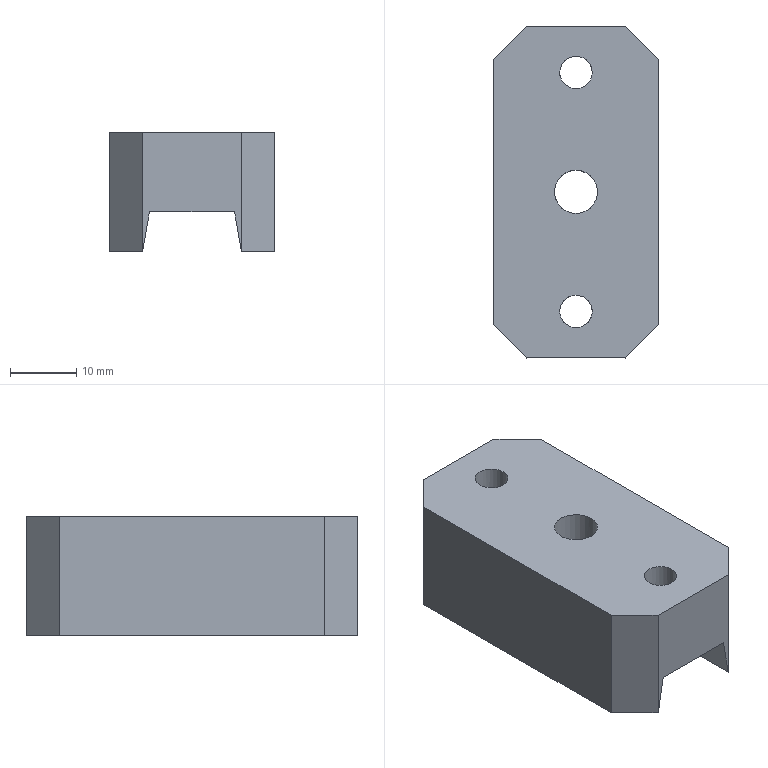Part | STEP file | 车灯-后视镜_id258_x_t | 1 solid | 19 faces | box 25 x 50 x 18 mm | volume 16008 mm3 | plane 15 | cylinder 4 | commonest cylinder face diameters 4.9 x2 6.5 x1 12.5 x1
STEP:
#1=CARTESIAN_POINT('',(-180.,153.25,17.94));
#2=VERTEX_POINT('',#1);
#3=CARTESIAN_POINT('',(-180.,150.,17.94));
#4=DIRECTION('',(0.,0.,-1.));
#5=DIRECTION('',(0.,1.,0.));
#6=AXIS2_PLACEMENT_3D('',#3,#4,#5);
#7=CIRCLE('',#6,3.25);
#8=EDGE_CURVE('',#2,#2,#7,.T.);
#9=ORIENTED_EDGE('',*,*,#8,.F.);
#10=EDGE_LOOP('',(#9));
#11=FACE_BOUND('',#10,.T.);
#12=CARTESIAN_POINT('',(-183.25,150.,12.44));
#13=VERTEX_POINT('',#12);
#14=CARTESIAN_POINT('',(-180.,150.,12.44));
#15=DIRECTION('',(0.,0.,1.));
#16=DIRECTION('',(-1.,0.,0.));
#17=AXIS2_PLACEMENT_3D('',#14,#15,#16);
#18=CIRCLE('',#17,3.25);
#19=EDGE_CURVE('',#13,#13,#18,.T.);
#20=ORIENTED_EDGE('',*,*,#19,.F.);
#21=EDGE_LOOP('',(#20));
#22=FACE_BOUND('',#21,.T.);
#23=CARTESIAN_POINT('',(-180.,150.,21.94));
#24=DIRECTION('',(0.,0.,-1.));
#25=DIRECTION('',(1.,0.,0.));
#26=AXIS2_PLACEMENT_3D('',#23,#24,#25);
#27=CYLINDRICAL_SURFACE('',#26,3.25);
#28=ADVANCED_FACE('',(#11,#22),#27,.F.);
#29=CARTESIAN_POINT('',(-172.5,125.,17.94));
#30=VERTEX_POINT('',#29);
#31=CARTESIAN_POINT('',(-187.5,125.,17.94));
#32=VERTEX_POINT('',#31);
#33=CARTESIAN_POINT('',(-195.,125.,17.94));
#34=DIRECTION('',(-1.,0.,0.));
#35=VECTOR('',#34,1.);
#36=LINE('',#33,#35);
#37=EDGE_CURVE('',#30,#32,#36,.T.);
#38=ORIENTED_EDGE('',*,*,#37,.T.);
#39=CARTESIAN_POINT('',(-187.5,125.,-0.05985));
#40=VERTEX_POINT('',#39);
#41=CARTESIAN_POINT('',(-187.5,125.,-0.05985));
#42=DIRECTION('',(0.,0.,-1.));
#43=VECTOR('',#42,1.);
#44=LINE('',#41,#43);
#45=EDGE_CURVE('',#32,#40,#44,.T.);
#46=ORIENTED_EDGE('',*,*,#45,.T.);
#47=CARTESIAN_POINT('',(-187.461,125.,-0.05985));
#48=VERTEX_POINT('',#47);
#49=CARTESIAN_POINT('',(-195.,125.,-0.05985));
#50=DIRECTION('',(-1.,0.,0.));
#51=VECTOR('',#50,1.);
#52=LINE('',#49,#51);
#53=EDGE_CURVE('',#48,#40,#52,.T.);
#54=ORIENTED_EDGE('',*,*,#53,.F.);
#55=CARTESIAN_POINT('',(-186.403,125.,5.94));
#56=VERTEX_POINT('',#55);
#57=CARTESIAN_POINT('',(-187.538,125.,-0.494));
#58=DIRECTION('',(-0.1736,0.,-0.9848));
#59=VECTOR('',#58,1.);
#60=LINE('',#57,#59);
#61=EDGE_CURVE('',#56,#48,#60,.T.);
#62=ORIENTED_EDGE('',*,*,#61,.F.);
#63=CARTESIAN_POINT('',(-173.597,125.,5.94));
#64=VERTEX_POINT('',#63);
#65=CARTESIAN_POINT('',(-172.5,125.,5.94));
#66=DIRECTION('',(-1.,0.,0.));
#67=VECTOR('',#66,1.);
#68=LINE('',#65,#67);
#69=EDGE_CURVE('',#64,#56,#68,.T.);
#70=ORIENTED_EDGE('',*,*,#69,.F.);
#71=CARTESIAN_POINT('',(-172.539,125.,-0.05985));
#72=VERTEX_POINT('',#71);
#73=CARTESIAN_POINT('',(-172.462,125.,-0.494));
#74=DIRECTION('',(0.1736,0.,-0.9848));
#75=VECTOR('',#74,1.);
#76=LINE('',#73,#75);
#77=EDGE_CURVE('',#64,#72,#76,.T.);
#78=ORIENTED_EDGE('',*,*,#77,.T.);
#79=CARTESIAN_POINT('',(-172.5,125.,-0.05985));
#80=VERTEX_POINT('',#79);
#81=CARTESIAN_POINT('',(-195.,125.,-0.05985));
#82=DIRECTION('',(-1.,0.,0.));
#83=VECTOR('',#82,1.);
#84=LINE('',#81,#83);
#85=EDGE_CURVE('',#80,#72,#84,.T.);
#86=ORIENTED_EDGE('',*,*,#85,.F.);
#87=CARTESIAN_POINT('',(-172.5,125.,-0.05985));
#88=DIRECTION('',(0.,0.,1.));
#89=VECTOR('',#88,1.);
#90=LINE('',#87,#89);
#91=EDGE_CURVE('',#80,#30,#90,.T.);
#92=ORIENTED_EDGE('',*,*,#91,.T.);
#93=EDGE_LOOP('',(#38,#46,#54,#62,#70,#78,#86,#92));
#94=FACE_OUTER_BOUND('',#93,.T.);
#95=CARTESIAN_POINT('',(-165.,125.,-0.05985));
#96=DIRECTION('',(0.,1.,0.));
#97=DIRECTION('',(1.,0.,0.));
#98=AXIS2_PLACEMENT_3D('',#95,#96,#97);
#99=PLANE('',#98);
#100=ADVANCED_FACE('',(#94),#99,.F.);
#101=CARTESIAN_POINT('',(-172.5,175.,17.94));
#102=VERTEX_POINT('',#101);
#103=CARTESIAN_POINT('',(-187.5,175.,17.94));
#104=VERTEX_POINT('',#103);
#105=CARTESIAN_POINT('',(-195.,175.,17.94));
#106=DIRECTION('',(-1.,0.,0.));
#107=VECTOR('',#106,1.);
#108=LINE('',#105,#107);
#109=EDGE_CURVE('',#102,#104,#108,.T.);
#110=ORIENTED_EDGE('',*,*,#109,.F.);
#111=CARTESIAN_POINT('',(-172.5,175.,-0.05985));
#112=VERTEX_POINT('',#111);
#113=CARTESIAN_POINT('',(-172.5,175.,-0.05985));
#114=DIRECTION('',(0.,0.,-1.));
#115=VECTOR('',#114,1.);
#116=LINE('',#113,#115);
#117=EDGE_CURVE('',#102,#112,#116,.T.);
#118=ORIENTED_EDGE('',*,*,#117,.T.);
#119=CARTESIAN_POINT('',(-172.539,175.,-0.05985));
#120=VERTEX_POINT('',#119);
#121=CARTESIAN_POINT('',(-195.,175.,-0.05985));
#122=DIRECTION('',(-1.,0.,0.));
#123=VECTOR('',#122,1.);
#124=LINE('',#121,#123);
#125=EDGE_CURVE('',#112,#120,#124,.T.);
#126=ORIENTED_EDGE('',*,*,#125,.T.);
#127=CARTESIAN_POINT('',(-173.597,175.,5.94));
#128=VERTEX_POINT('',#127);
#129=CARTESIAN_POINT('',(-172.462,175.,-0.494));
#130=DIRECTION('',(0.1736,0.,-0.9848));
#131=VECTOR('',#130,1.);
#132=LINE('',#129,#131);
#133=EDGE_CURVE('',#128,#120,#132,.T.);
#134=ORIENTED_EDGE('',*,*,#133,.F.);
#135=CARTESIAN_POINT('',(-186.403,175.,5.94));
#136=VERTEX_POINT('',#135);
#137=CARTESIAN_POINT('',(-172.5,175.,5.94));
#138=DIRECTION('',(-1.,0.,0.));
#139=VECTOR('',#138,1.);
#140=LINE('',#137,#139);
#141=EDGE_CURVE('',#128,#136,#140,.T.);
#142=ORIENTED_EDGE('',*,*,#141,.T.);
#143=CARTESIAN_POINT('',(-187.461,175.,-0.05985));
#144=VERTEX_POINT('',#143);
#145=CARTESIAN_POINT('',(-187.538,175.,-0.494));
#146=DIRECTION('',(-0.1736,0.,-0.9848));
#147=VECTOR('',#146,1.);
#148=LINE('',#145,#147);
#149=EDGE_CURVE('',#136,#144,#148,.T.);
#150=ORIENTED_EDGE('',*,*,#149,.T.);
#151=CARTESIAN_POINT('',(-187.5,175.,-0.05985));
#152=VERTEX_POINT('',#151);
#153=CARTESIAN_POINT('',(-195.,175.,-0.05985));
#154=DIRECTION('',(-1.,0.,0.));
#155=VECTOR('',#154,1.);
#156=LINE('',#153,#155);
#157=EDGE_CURVE('',#144,#152,#156,.T.);
#158=ORIENTED_EDGE('',*,*,#157,.T.);
#159=CARTESIAN_POINT('',(-187.5,175.,-0.05985));
#160=DIRECTION('',(0.,0.,1.));
#161=VECTOR('',#160,1.);
#162=LINE('',#159,#161);
#163=EDGE_CURVE('',#152,#104,#162,.T.);
#164=ORIENTED_EDGE('',*,*,#163,.T.);
#165=EDGE_LOOP('',(#110,#118,#126,#134,#142,#150,#158,#164));
#166=FACE_OUTER_BOUND('',#165,.T.);
#167=CARTESIAN_POINT('',(-165.,175.,-0.05985));
#168=DIRECTION('',(0.,1.,0.));
#169=DIRECTION('',(1.,0.,0.));
#170=AXIS2_PLACEMENT_3D('',#167,#168,#169);
#171=PLANE('',#170);
#172=ADVANCED_FACE('',(#166),#171,.T.);
#173=ORIENTED_EDGE('',*,*,#125,.F.);
#174=CARTESIAN_POINT('',(-167.5,170.,-0.05985));
#175=VERTEX_POINT('',#174);
#176=CARTESIAN_POINT('',(-172.5,175.,-0.05985));
#177=DIRECTION('',(0.7071,-0.7071,0.));
#178=VECTOR('',#177,1.);
#179=LINE('',#176,#178);
#180=EDGE_CURVE('',#112,#175,#179,.T.);
#181=ORIENTED_EDGE('',*,*,#180,.T.);
#182=CARTESIAN_POINT('',(-167.5,130.,-0.05985));
#183=VERTEX_POINT('',#182);
#184=CARTESIAN_POINT('',(-167.5,100.,-0.05985));
#185=DIRECTION('',(0.,-1.,0.));
#186=VECTOR('',#185,1.);
#187=LINE('',#184,#186);
#188=EDGE_CURVE('',#175,#183,#187,.T.);
#189=ORIENTED_EDGE('',*,*,#188,.T.);
#190=CARTESIAN_POINT('',(-167.5,130.,-0.05985));
#191=DIRECTION('',(-0.7071,-0.7071,0.));
#192=VECTOR('',#191,1.);
#193=LINE('',#190,#192);
#194=EDGE_CURVE('',#183,#80,#193,.T.);
#195=ORIENTED_EDGE('',*,*,#194,.T.);
#196=ORIENTED_EDGE('',*,*,#85,.T.);
#197=CARTESIAN_POINT('',(-172.539,150.,-0.05985));
#198=DIRECTION('',(0.,1.,0.));
#199=VECTOR('',#198,1.);
#200=LINE('',#197,#199);
#201=EDGE_CURVE('',#72,#120,#200,.T.);
#202=ORIENTED_EDGE('',*,*,#201,.T.);
#203=EDGE_LOOP('',(#173,#181,#189,#195,#196,#202));
#204=FACE_OUTER_BOUND('',#203,.T.);
#205=CARTESIAN_POINT('',(-195.,100.,-0.05985));
#206=DIRECTION('',(0.,0.,1.));
#207=DIRECTION('',(0.,-1.,0.));
#208=AXIS2_PLACEMENT_3D('',#205,#206,#207);
#209=PLANE('',#208);
#210=ADVANCED_FACE('',(#204),#209,.F.);
#211=CARTESIAN_POINT('',(-192.5,170.,17.94));
#212=VERTEX_POINT('',#211);
#213=CARTESIAN_POINT('',(-192.5,130.,17.94));
#214=VERTEX_POINT('',#213);
#215=CARTESIAN_POINT('',(-192.5,100.,17.94));
#216=DIRECTION('',(0.,-1.,0.));
#217=VECTOR('',#216,1.);
#218=LINE('',#215,#217);
#219=EDGE_CURVE('',#212,#214,#218,.T.);
#220=ORIENTED_EDGE('',*,*,#219,.F.);
#221=CARTESIAN_POINT('',(-192.5,170.,-0.05985));
#222=VERTEX_POINT('',#221);
#223=CARTESIAN_POINT('',(-192.5,170.,-0.05985));
#224=DIRECTION('',(0.,0.,-1.));
#225=VECTOR('',#224,1.);
#226=LINE('',#223,#225);
#227=EDGE_CURVE('',#212,#222,#226,.T.);
#228=ORIENTED_EDGE('',*,*,#227,.T.);
#229=CARTESIAN_POINT('',(-192.5,130.,-0.05985));
#230=VERTEX_POINT('',#229);
#231=CARTESIAN_POINT('',(-192.5,100.,-0.05985));
#232=DIRECTION('',(0.,-1.,0.));
#233=VECTOR('',#232,1.);
#234=LINE('',#231,#233);
#235=EDGE_CURVE('',#222,#230,#234,.T.);
#236=ORIENTED_EDGE('',*,*,#235,.T.);
#237=CARTESIAN_POINT('',(-192.5,130.,17.94));
#238=DIRECTION('',(0.,0.,1.));
#239=VECTOR('',#238,1.);
#240=LINE('',#237,#239);
#241=EDGE_CURVE('',#230,#214,#240,.T.);
#242=ORIENTED_EDGE('',*,*,#241,.T.);
#243=EDGE_LOOP('',(#220,#228,#236,#242));
#244=FACE_OUTER_BOUND('',#243,.T.);
#245=CARTESIAN_POINT('',(-192.5,200.,-0.05985));
#246=DIRECTION('',(-1.,0.,0.));
#247=DIRECTION('',(0.,1.,0.));
#248=AXIS2_PLACEMENT_3D('',#245,#246,#247);
#249=PLANE('',#248);
#250=ADVANCED_FACE('',(#244),#249,.T.);
#251=ORIENTED_EDGE('',*,*,#188,.F.);
#252=CARTESIAN_POINT('',(-167.5,170.,17.94));
#253=VERTEX_POINT('',#252);
#254=CARTESIAN_POINT('',(-167.5,170.,17.94));
#255=DIRECTION('',(0.,0.,1.));
#256=VECTOR('',#255,1.);
#257=LINE('',#254,#256);
#258=EDGE_CURVE('',#175,#253,#257,.T.);
#259=ORIENTED_EDGE('',*,*,#258,.T.);
#260=CARTESIAN_POINT('',(-167.5,130.,17.94));
#261=VERTEX_POINT('',#260);
#262=CARTESIAN_POINT('',(-167.5,100.,17.94));
#263=DIRECTION('',(0.,-1.,0.));
#264=VECTOR('',#263,1.);
#265=LINE('',#262,#264);
#266=EDGE_CURVE('',#253,#261,#265,.T.);
#267=ORIENTED_EDGE('',*,*,#266,.T.);
#268=CARTESIAN_POINT('',(-167.5,130.,-0.05985));
#269=DIRECTION('',(0.,0.,-1.));
#270=VECTOR('',#269,1.);
#271=LINE('',#268,#270);
#272=EDGE_CURVE('',#261,#183,#271,.T.);
#273=ORIENTED_EDGE('',*,*,#272,.T.);
#274=EDGE_LOOP('',(#251,#259,#267,#273));
#275=FACE_OUTER_BOUND('',#274,.T.);
#276=CARTESIAN_POINT('',(-167.5,200.,-0.05985));
#277=DIRECTION('',(-1.,0.,0.));
#278=DIRECTION('',(0.,1.,0.));
#279=AXIS2_PLACEMENT_3D('',#276,#277,#278);
#280=PLANE('',#279);
#281=ADVANCED_FACE('',(#275),#280,.F.);
#282=ORIENTED_EDGE('',*,*,#235,.F.);
#283=CARTESIAN_POINT('',(-192.5,170.,-0.05985));
#284=DIRECTION('',(0.7071,0.7071,0.));
#285=VECTOR('',#284,1.);
#286=LINE('',#283,#285);
#287=EDGE_CURVE('',#222,#152,#286,.T.);
#288=ORIENTED_EDGE('',*,*,#287,.T.);
#289=ORIENTED_EDGE('',*,*,#157,.F.);
#290=CARTESIAN_POINT('',(-187.461,150.,-0.05985));
#291=DIRECTION('',(0.,1.,0.));
#292=VECTOR('',#291,1.);
#293=LINE('',#290,#292);
#294=EDGE_CURVE('',#48,#144,#293,.T.);
#295=ORIENTED_EDGE('',*,*,#294,.F.);
#296=ORIENTED_EDGE('',*,*,#53,.T.);
#297=CARTESIAN_POINT('',(-187.5,125.,-0.05985));
#298=DIRECTION('',(-0.7071,0.7071,0.));
#299=VECTOR('',#298,1.);
#300=LINE('',#297,#299);
#301=EDGE_CURVE('',#40,#230,#300,.T.);
#302=ORIENTED_EDGE('',*,*,#301,.T.);
#303=EDGE_LOOP('',(#282,#288,#289,#295,#296,#302));
#304=FACE_OUTER_BOUND('',#303,.T.);
#305=CARTESIAN_POINT('',(-195.,100.,-0.05985));
#306=DIRECTION('',(0.,0.,1.));
#307=DIRECTION('',(0.,-1.,0.));
#308=AXIS2_PLACEMENT_3D('',#305,#306,#307);
#309=PLANE('',#308);
#310=ADVANCED_FACE('',(#304),#309,.F.);
#311=ORIENTED_EDGE('',*,*,#266,.F.);
#312=CARTESIAN_POINT('',(-146.25,148.75,17.94));
#313=DIRECTION('',(-0.7071,0.7071,0.));
#314=VECTOR('',#313,1.);
#315=LINE('',#312,#314);
#316=EDGE_CURVE('',#253,#102,#315,.T.);
#317=ORIENTED_EDGE('',*,*,#316,.T.);
#318=ORIENTED_EDGE('',*,*,#109,.T.);
#319=CARTESIAN_POINT('',(-228.75,133.75,17.94));
#320=DIRECTION('',(-0.7071,-0.7071,0.));
#321=VECTOR('',#320,1.);
#322=LINE('',#319,#321);
#323=EDGE_CURVE('',#104,#212,#322,.T.);
#324=ORIENTED_EDGE('',*,*,#323,.T.);
#325=ORIENTED_EDGE('',*,*,#219,.T.);
#326=CARTESIAN_POINT('',(-178.75,116.25,17.94));
#327=DIRECTION('',(0.7071,-0.7071,0.));
#328=VECTOR('',#327,1.);
#329=LINE('',#326,#328);
#330=EDGE_CURVE('',#214,#32,#329,.T.);
#331=ORIENTED_EDGE('',*,*,#330,.T.);
#332=ORIENTED_EDGE('',*,*,#37,.F.);
#333=CARTESIAN_POINT('',(-196.25,101.25,17.94));
#334=DIRECTION('',(0.7071,0.7071,0.));
#335=VECTOR('',#334,1.);
#336=LINE('',#333,#335);
#337=EDGE_CURVE('',#30,#261,#336,.T.);
#338=ORIENTED_EDGE('',*,*,#337,.T.);
#339=EDGE_LOOP('',(#311,#317,#318,#324,#325,#331,#332,#338));
#340=FACE_BOUND('',#339,.T.);
#341=CARTESIAN_POINT('',(-180.,170.45,17.94));
#342=VERTEX_POINT('',#341);
#343=CARTESIAN_POINT('',(-180.,168.,17.94));
#344=DIRECTION('',(0.,0.,-1.));
#345=DIRECTION('',(0.,1.,0.));
#346=AXIS2_PLACEMENT_3D('',#343,#344,#345);
#347=CIRCLE('',#346,2.45);
#348=EDGE_CURVE('',#342,#342,#347,.T.);
#349=ORIENTED_EDGE('',*,*,#348,.T.);
#350=EDGE_LOOP('',(#349));
#351=FACE_BOUND('',#350,.T.);
#352=ORIENTED_EDGE('',*,*,#8,.T.);
#353=EDGE_LOOP('',(#352));
#354=FACE_BOUND('',#353,.T.);
#355=CARTESIAN_POINT('',(-180.,134.45,17.94));
#356=VERTEX_POINT('',#355);
#357=CARTESIAN_POINT('',(-180.,132.,17.94));
#358=DIRECTION('',(0.,0.,-1.));
#359=DIRECTION('',(0.,1.,0.));
#360=AXIS2_PLACEMENT_3D('',#357,#358,#359);
#361=CIRCLE('',#360,2.45);
#362=EDGE_CURVE('',#356,#356,#361,.T.);
#363=ORIENTED_EDGE('',*,*,#362,.T.);
#364=EDGE_LOOP('',(#363));
#365=FACE_BOUND('',#364,.T.);
#366=CARTESIAN_POINT('',(-195.,100.,17.94));
#367=DIRECTION('',(0.,0.,1.));
#368=DIRECTION('',(0.,-1.,0.));
#369=AXIS2_PLACEMENT_3D('',#366,#367,#368);
#370=PLANE('',#369);
#371=ADVANCED_FACE('',(#340,#351,#354,#365),#370,.T.);
#372=CARTESIAN_POINT('',(-177.55,168.,5.94));
#373=VERTEX_POINT('',#372);
#374=CARTESIAN_POINT('',(-180.,168.,5.94));
#375=DIRECTION('',(0.,0.,-1.));
#376=DIRECTION('',(1.,0.,0.));
#377=AXIS2_PLACEMENT_3D('',#374,#375,#376);
#378=CIRCLE('',#377,2.45);
#379=EDGE_CURVE('',#373,#373,#378,.T.);
#380=ORIENTED_EDGE('',*,*,#379,.T.);
#381=EDGE_LOOP('',(#380));
#382=FACE_BOUND('',#381,.T.);
#383=ORIENTED_EDGE('',*,*,#348,.F.);
#384=EDGE_LOOP('',(#383));
#385=FACE_BOUND('',#384,.T.);
#386=CARTESIAN_POINT('',(-180.,168.,21.94));
#387=DIRECTION('',(0.,0.,-1.));
#388=DIRECTION('',(1.,0.,0.));
#389=AXIS2_PLACEMENT_3D('',#386,#387,#388);
#390=CYLINDRICAL_SURFACE('',#389,2.45);
#391=ADVANCED_FACE('',(#382,#385),#390,.F.);
#392=ORIENTED_EDGE('',*,*,#379,.F.);
#393=EDGE_LOOP('',(#392));
#394=FACE_BOUND('',#393,.T.);
#395=CARTESIAN_POINT('',(-173.597,150.,5.94));
#396=DIRECTION('',(0.,1.,0.));
#397=VECTOR('',#396,1.);
#398=LINE('',#395,#397);
#399=EDGE_CURVE('',#64,#128,#398,.T.);
#400=ORIENTED_EDGE('',*,*,#399,.F.);
#401=ORIENTED_EDGE('',*,*,#69,.T.);
#402=CARTESIAN_POINT('',(-186.403,150.,5.94));
#403=DIRECTION('',(0.,1.,0.));
#404=VECTOR('',#403,1.);
#405=LINE('',#402,#404);
#406=EDGE_CURVE('',#56,#136,#405,.T.);
#407=ORIENTED_EDGE('',*,*,#406,.T.);
#408=ORIENTED_EDGE('',*,*,#141,.F.);
#409=EDGE_LOOP('',(#400,#401,#407,#408));
#410=FACE_BOUND('',#409,.T.);
#411=CARTESIAN_POINT('',(-186.25,150.,5.94));
#412=VERTEX_POINT('',#411);
#413=CARTESIAN_POINT('',(-180.,150.,5.94));
#414=DIRECTION('',(0.,0.,1.));
#415=DIRECTION('',(-1.,0.,0.));
#416=AXIS2_PLACEMENT_3D('',#413,#414,#415);
#417=CIRCLE('',#416,6.25);
#418=EDGE_CURVE('',#412,#412,#417,.T.);
#419=ORIENTED_EDGE('',*,*,#418,.T.);
#420=EDGE_LOOP('',(#419));
#421=FACE_BOUND('',#420,.T.);
#422=CARTESIAN_POINT('',(-177.55,132.,5.94));
#423=VERTEX_POINT('',#422);
#424=CARTESIAN_POINT('',(-180.,132.,5.94));
#425=DIRECTION('',(0.,0.,-1.));
#426=DIRECTION('',(1.,0.,0.));
#427=AXIS2_PLACEMENT_3D('',#424,#425,#426);
#428=CIRCLE('',#427,2.45);
#429=EDGE_CURVE('',#423,#423,#428,.T.);
#430=ORIENTED_EDGE('',*,*,#429,.F.);
#431=EDGE_LOOP('',(#430));
#432=FACE_BOUND('',#431,.T.);
#433=CARTESIAN_POINT('',(-172.5,125.,5.94));
#434=DIRECTION('',(0.,0.,1.));
#435=DIRECTION('',(-1.,0.,0.));
#436=AXIS2_PLACEMENT_3D('',#433,#434,#435);
#437=PLANE('',#436);
#438=ADVANCED_FACE('',(#394,#410,#421,#432),#437,.F.);
#439=ORIENTED_EDGE('',*,*,#201,.F.);
#440=ORIENTED_EDGE('',*,*,#77,.F.);
#441=ORIENTED_EDGE('',*,*,#399,.T.);
#442=ORIENTED_EDGE('',*,*,#133,.T.);
#443=EDGE_LOOP('',(#439,#440,#441,#442));
#444=FACE_OUTER_BOUND('',#443,.T.);
#445=CARTESIAN_POINT('',(-172.462,150.,-0.494));
#446=DIRECTION('',(-0.9848,0.,-0.1736));
#447=DIRECTION('',(0.1736,0.,-0.9848));
#448=AXIS2_PLACEMENT_3D('',#445,#446,#447);
#449=PLANE('',#448);
#450=ADVANCED_FACE('',(#444),#449,.T.);
#451=ORIENTED_EDGE('',*,*,#294,.T.);
#452=ORIENTED_EDGE('',*,*,#149,.F.);
#453=ORIENTED_EDGE('',*,*,#406,.F.);
#454=ORIENTED_EDGE('',*,*,#61,.T.);
#455=EDGE_LOOP('',(#451,#452,#453,#454));
#456=FACE_OUTER_BOUND('',#455,.T.);
#457=CARTESIAN_POINT('',(-187.538,150.,-0.494));
#458=DIRECTION('',(0.9848,0.,-0.1736));
#459=DIRECTION('',(0.1736,0.,0.9848));
#460=AXIS2_PLACEMENT_3D('',#457,#458,#459);
#461=PLANE('',#460);
#462=ADVANCED_FACE('',(#456),#461,.T.);
#463=CARTESIAN_POINT('',(-186.25,150.,12.44));
#464=VERTEX_POINT('',#463);
#465=CARTESIAN_POINT('',(-180.,150.,12.44));
#466=DIRECTION('',(0.,0.,1.));
#467=DIRECTION('',(-1.,0.,0.));
#468=AXIS2_PLACEMENT_3D('',#465,#466,#467);
#469=CIRCLE('',#468,6.25);
#470=EDGE_CURVE('',#464,#464,#469,.T.);
#471=ORIENTED_EDGE('',*,*,#470,.F.);
#472=EDGE_LOOP('',(#471));
#473=FACE_BOUND('',#472,.T.);
#474=ORIENTED_EDGE('',*,*,#19,.T.);
#475=EDGE_LOOP('',(#474));
#476=FACE_BOUND('',#475,.T.);
#477=CARTESIAN_POINT('',(-180.,150.,12.44));
#478=DIRECTION('',(0.,0.,-1.));
#479=DIRECTION('',(1.,0.,0.));
#480=AXIS2_PLACEMENT_3D('',#477,#478,#479);
#481=PLANE('',#480);
#482=ADVANCED_FACE('',(#473,#476),#481,.T.);
#483=ORIENTED_EDGE('',*,*,#470,.T.);
#484=EDGE_LOOP('',(#483));
#485=FACE_BOUND('',#484,.T.);
#486=ORIENTED_EDGE('',*,*,#418,.F.);
#487=EDGE_LOOP('',(#486));
#488=FACE_BOUND('',#487,.T.);
#489=CARTESIAN_POINT('',(-180.,150.,5.94));
#490=DIRECTION('',(0.,0.,1.));
#491=DIRECTION('',(-1.,0.,0.));
#492=AXIS2_PLACEMENT_3D('',#489,#490,#491);
#493=CYLINDRICAL_SURFACE('',#492,6.25);
#494=ADVANCED_FACE('',(#485,#488),#493,.F.);
#495=ORIENTED_EDGE('',*,*,#362,.F.);
#496=EDGE_LOOP('',(#495));
#497=FACE_BOUND('',#496,.T.);
#498=ORIENTED_EDGE('',*,*,#429,.T.);
#499=EDGE_LOOP('',(#498));
#500=FACE_BOUND('',#499,.T.);
#501=CARTESIAN_POINT('',(-180.,132.,5.94));
#502=DIRECTION('',(0.,0.,1.));
#503=DIRECTION('',(-1.,0.,0.));
#504=AXIS2_PLACEMENT_3D('',#501,#502,#503);
#505=CYLINDRICAL_SURFACE('',#504,2.45);
#506=ADVANCED_FACE('',(#497,#500),#505,.F.);
#507=ORIENTED_EDGE('',*,*,#316,.F.);
#508=ORIENTED_EDGE('',*,*,#258,.F.);
#509=ORIENTED_EDGE('',*,*,#180,.F.);
#510=ORIENTED_EDGE('',*,*,#117,.F.);
#511=EDGE_LOOP('',(#507,#508,#509,#510));
#512=FACE_OUTER_BOUND('',#511,.T.);
#513=CARTESIAN_POINT('',(-172.5,175.,-0.05985));
#514=DIRECTION('',(0.7071,0.7071,0.));
#515=DIRECTION('',(0.7071,-0.7071,0.));
#516=AXIS2_PLACEMENT_3D('',#513,#514,#515);
#517=PLANE('',#516);
#518=ADVANCED_FACE('',(#512),#517,.T.);
#519=ORIENTED_EDGE('',*,*,#323,.F.);
#520=ORIENTED_EDGE('',*,*,#163,.F.);
#521=ORIENTED_EDGE('',*,*,#287,.F.);
#522=ORIENTED_EDGE('',*,*,#227,.F.);
#523=EDGE_LOOP('',(#519,#520,#521,#522));
#524=FACE_OUTER_BOUND('',#523,.T.);
#525=CARTESIAN_POINT('',(-192.5,170.,-0.05985));
#526=DIRECTION('',(0.7071,-0.7071,0.));
#527=DIRECTION('',(-0.7071,-0.7071,0.));
#528=AXIS2_PLACEMENT_3D('',#525,#526,#527);
#529=PLANE('',#528);
#530=ADVANCED_FACE('',(#524),#529,.F.);
#531=ORIENTED_EDGE('',*,*,#330,.F.);
#532=ORIENTED_EDGE('',*,*,#241,.F.);
#533=ORIENTED_EDGE('',*,*,#301,.F.);
#534=ORIENTED_EDGE('',*,*,#45,.F.);
#535=EDGE_LOOP('',(#531,#532,#533,#534));
#536=FACE_OUTER_BOUND('',#535,.T.);
#537=CARTESIAN_POINT('',(-187.5,125.,-0.05985));
#538=DIRECTION('',(-0.7071,-0.7071,0.));
#539=DIRECTION('',(-0.7071,0.7071,0.));
#540=AXIS2_PLACEMENT_3D('',#537,#538,#539);
#541=PLANE('',#540);
#542=ADVANCED_FACE('',(#536),#541,.T.);
#543=ORIENTED_EDGE('',*,*,#337,.F.);
#544=ORIENTED_EDGE('',*,*,#91,.F.);
#545=ORIENTED_EDGE('',*,*,#194,.F.);
#546=ORIENTED_EDGE('',*,*,#272,.F.);
#547=EDGE_LOOP('',(#543,#544,#545,#546));
#548=FACE_OUTER_BOUND('',#547,.T.);
#549=CARTESIAN_POINT('',(-167.5,130.,-0.05985));
#550=DIRECTION('',(-0.7071,0.7071,0.));
#551=DIRECTION('',(0.7071,0.7071,0.));
#552=AXIS2_PLACEMENT_3D('',#549,#550,#551);
#553=PLANE('',#552);
#554=ADVANCED_FACE('',(#548),#553,.F.);
#555=CLOSED_SHELL('',(#28,#100,#172,#210,#250,#281,#310,#371,#391,#438,#450,#462,#482,#494,#506,#518,#530,#542,#554));
#556=MANIFOLD_SOLID_BREP('',#555);
#557=(LENGTH_UNIT()NAMED_UNIT(*)SI_UNIT(.MILLI.,.METRE.));
#558=UNCERTAINTY_MEASURE_WITH_UNIT(LENGTH_MEASURE(0.00002),#557,'','');
#559=(NAMED_UNIT(*)PLANE_ANGLE_UNIT()SI_UNIT($,.RADIAN.));
#560=PLANE_ANGLE_MEASURE_WITH_UNIT(PLANE_ANGLE_MEASURE(0.01745),#559);
#561=DIMENSIONAL_EXPONENTS(0.,0.,0.,0.,0.,0.,0.);
#562=(CONVERSION_BASED_UNIT('DEGREE',#560)NAMED_UNIT(#561)PLANE_ANGLE_UNIT());
#563=(NAMED_UNIT(*)SI_UNIT($,.STERADIAN.)SOLID_ANGLE_UNIT());
#564=(GEOMETRIC_REPRESENTATION_CONTEXT(3)GLOBAL_UNCERTAINTY_ASSIGNED_CONTEXT((#558))GLOBAL_UNIT_ASSIGNED_CONTEXT((#557,#562,#563))REPRESENTATION_CONTEXT('',''));
#565=ADVANCED_BREP_SHAPE_REPRESENTATION('',(#556),#564);